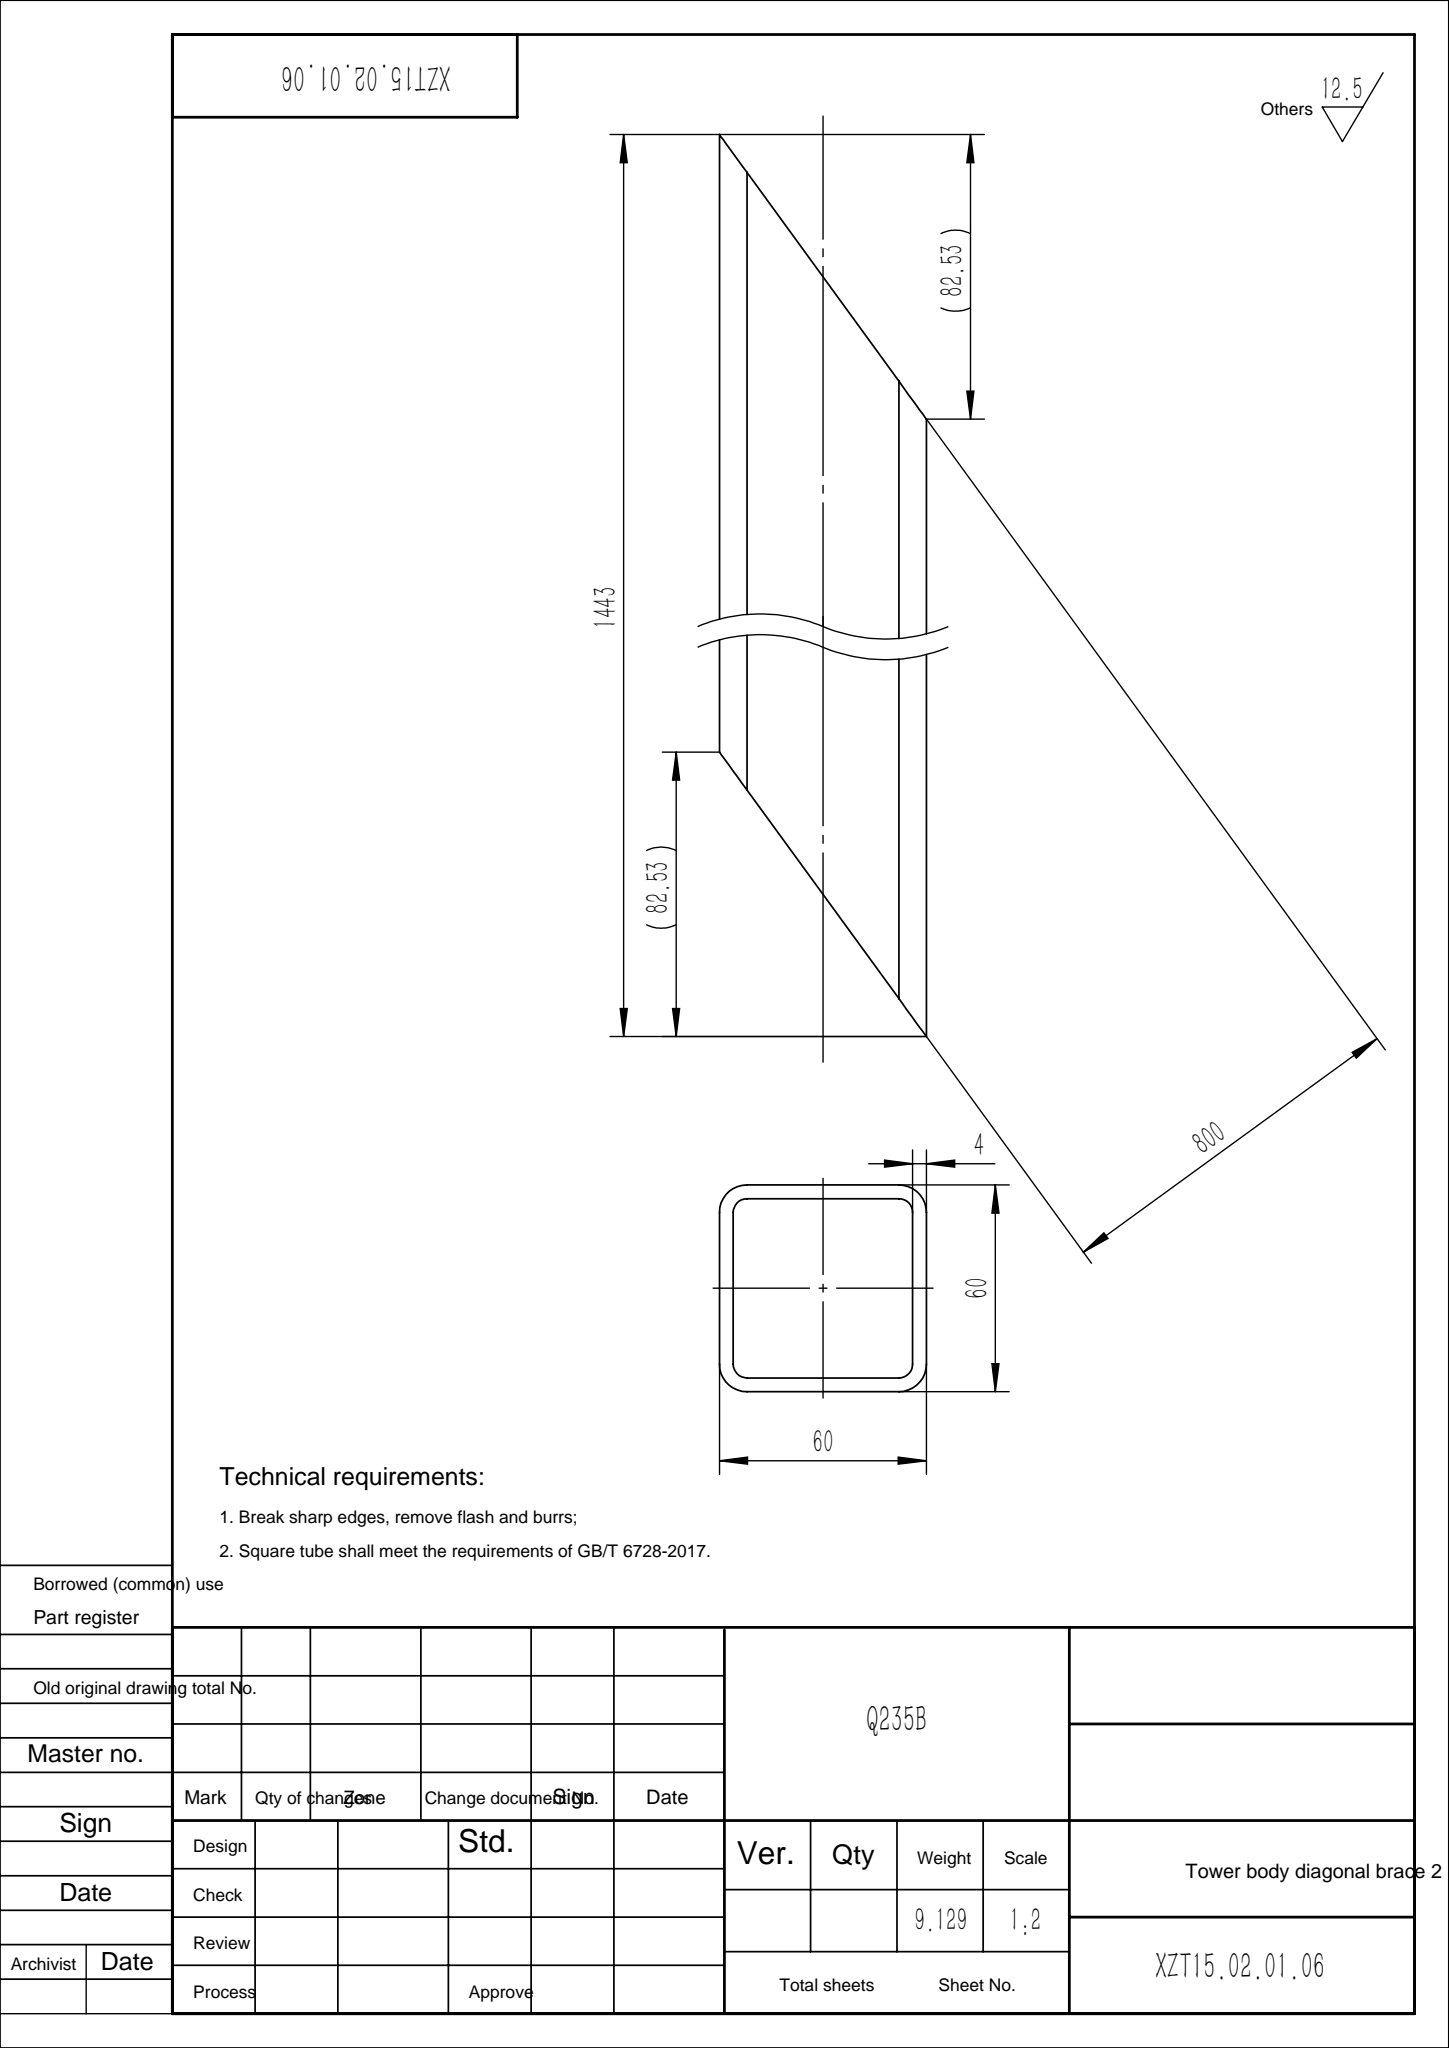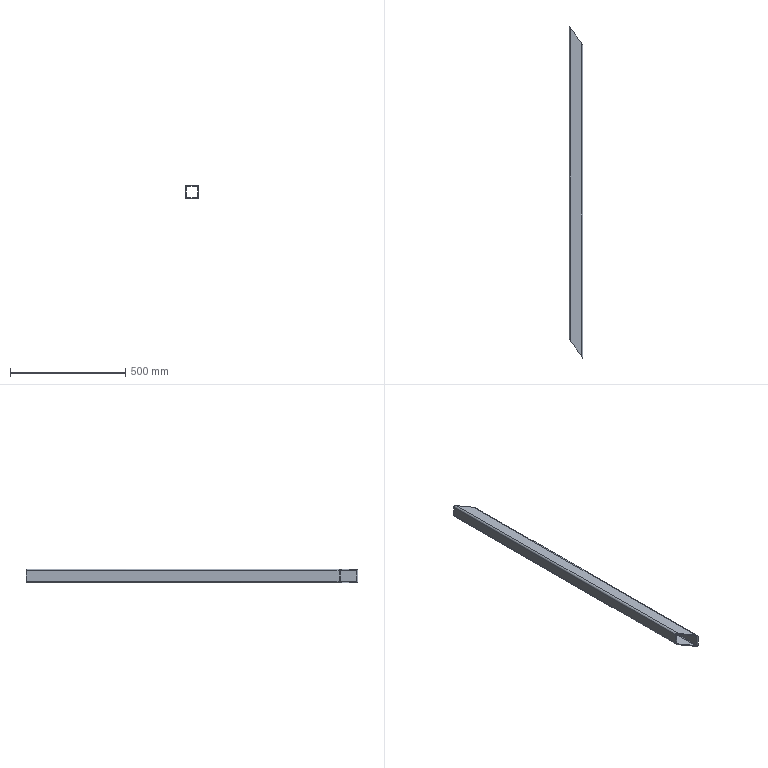Part | SolidWorks | features ICE 1, WeldMemberFeat 1, WeldmentFeature 1 | 1 solid | 18 faces | box 60 x 1443 x 60 mm | volume 1162925 mm3 | plane 10 | cylinder 8 | commonest cylinder face diameters 8 x4 16 x4
STEP:
#1=CARTESIAN_POINT('',(30.,1360.47,-22.));
#2=VERTEX_POINT('',#1);
#3=CARTESIAN_POINT('',(30.,0.,-22.));
#4=VERTEX_POINT('',#3);
#5=CARTESIAN_POINT('',(30.,1443.,-22.));
#6=DIRECTION('',(0.,-1.,0.));
#7=VECTOR('',#6,1000.);
#8=LINE('',#5,#7);
#9=EDGE_CURVE('',#2,#4,#8,.T.);
#10=ORIENTED_EDGE('',*,*,#9,.F.);
#11=CARTESIAN_POINT('',(30.,1360.47,22.));
#12=VERTEX_POINT('',#11);
#13=CARTESIAN_POINT('',(30.,1360.47,-30.));
#14=DIRECTION('',(0.,0.,1.));
#15=VECTOR('',#14,1000.);
#16=LINE('',#13,#15);
#17=EDGE_CURVE('',#2,#12,#16,.T.);
#18=ORIENTED_EDGE('',*,*,#17,.T.);
#19=CARTESIAN_POINT('',(30.,0.,22.));
#20=VERTEX_POINT('',#19);
#21=CARTESIAN_POINT('',(30.,1443.,22.));
#22=DIRECTION('',(0.,-1.,0.));
#23=VECTOR('',#22,1000.);
#24=LINE('',#21,#23);
#25=EDGE_CURVE('',#12,#20,#24,.T.);
#26=ORIENTED_EDGE('',*,*,#25,.T.);
#27=CARTESIAN_POINT('',(30.,0.,-22.));
#28=DIRECTION('',(0.,0.,-1.));
#29=VECTOR('',#28,1000.);
#30=LINE('',#27,#29);
#31=EDGE_CURVE('',#20,#4,#30,.T.);
#32=ORIENTED_EDGE('',*,*,#31,.T.);
#33=EDGE_LOOP('',(#10,#18,#26,#32));
#34=FACE_OUTER_BOUND('',#33,.T.);
#35=CARTESIAN_POINT('',(30.,1443.,-22.));
#36=DIRECTION('',(-1.,0.,0.));
#37=DIRECTION('',(0.,0.,1.));
#38=AXIS2_PLACEMENT_3D('',#35,#36,#37);
#39=PLANE('',#38);
#40=ADVANCED_FACE('',(#34),#39,.F.);
#41=CARTESIAN_POINT('',(-30.,1443.,-22.));
#42=VERTEX_POINT('',#41);
#43=CARTESIAN_POINT('',(-30.,82.53,-22.));
#44=VERTEX_POINT('',#43);
#45=CARTESIAN_POINT('',(-30.,1443.,-22.));
#46=DIRECTION('',(0.,-1.,0.));
#47=VECTOR('',#46,1000.);
#48=LINE('',#45,#47);
#49=EDGE_CURVE('',#42,#44,#48,.T.);
#50=ORIENTED_EDGE('',*,*,#49,.T.);
#51=CARTESIAN_POINT('',(-30.,82.53,22.));
#52=VERTEX_POINT('',#51);
#53=CARTESIAN_POINT('',(-30.,82.53,-30.));
#54=DIRECTION('',(0.,0.,1.));
#55=VECTOR('',#54,1000.);
#56=LINE('',#53,#55);
#57=EDGE_CURVE('',#44,#52,#56,.T.);
#58=ORIENTED_EDGE('',*,*,#57,.T.);
#59=CARTESIAN_POINT('',(-30.,1443.,22.));
#60=VERTEX_POINT('',#59);
#61=CARTESIAN_POINT('',(-30.,1443.,22.));
#62=DIRECTION('',(0.,-1.,0.));
#63=VECTOR('',#62,1000.);
#64=LINE('',#61,#63);
#65=EDGE_CURVE('',#60,#52,#64,.T.);
#66=ORIENTED_EDGE('',*,*,#65,.F.);
#67=CARTESIAN_POINT('',(-30.,1443.,22.));
#68=DIRECTION('',(0.,0.,1.));
#69=VECTOR('',#68,1000.);
#70=LINE('',#67,#69);
#71=EDGE_CURVE('',#42,#60,#70,.T.);
#72=ORIENTED_EDGE('',*,*,#71,.F.);
#73=EDGE_LOOP('',(#50,#58,#66,#72));
#74=FACE_OUTER_BOUND('',#73,.T.);
#75=CARTESIAN_POINT('',(-30.,1443.,22.));
#76=DIRECTION('',(1.,0.,0.));
#77=DIRECTION('',(0.,0.,-1.));
#78=AXIS2_PLACEMENT_3D('',#75,#76,#77);
#79=PLANE('',#78);
#80=ADVANCED_FACE('',(#74),#79,.F.);
#81=ORIENTED_EDGE('',*,*,#49,.F.);
#82=CARTESIAN_POINT('',(-22.,1431.996,-30.));
#83=VERTEX_POINT('',#82);
#84=CARTESIAN_POINT('',(-30.,1443.,-22.));
#85=CARTESIAN_POINT('',(-30.,1443.,-26.686));
#86=CARTESIAN_POINT('',(-26.686,1438.442,-30.));
#87=CARTESIAN_POINT('',(-22.,1431.996,-30.));
#88=(BOUNDED_CURVE()B_SPLINE_CURVE(3,(#84,#85,#86,#87),.UNSPECIFIED.,.F.,.F.)B_SPLINE_CURVE_WITH_KNOTS((4,4),(3.142,4.712),.UNSPECIFIED.)CURVE()GEOMETRIC_REPRESENTATION_ITEM()RATIONAL_B_SPLINE_CURVE((1.,0.8047,0.8047,1.))REPRESENTATION_ITEM(''));
#89=EDGE_CURVE('',#42,#83,#88,.T.);
#90=ORIENTED_EDGE('',*,*,#89,.T.);
#91=CARTESIAN_POINT('',(-22.,71.526,-30.));
#92=VERTEX_POINT('',#91);
#93=CARTESIAN_POINT('',(-22.,1443.,-30.));
#94=DIRECTION('',(0.,-1.,0.));
#95=VECTOR('',#94,1000.);
#96=LINE('',#93,#95);
#97=EDGE_CURVE('',#83,#92,#96,.T.);
#98=ORIENTED_EDGE('',*,*,#97,.T.);
#99=CARTESIAN_POINT('',(-22.,71.526,-30.));
#100=CARTESIAN_POINT('',(-26.686,77.972,-30.));
#101=CARTESIAN_POINT('',(-30.,82.53,-26.686));
#102=CARTESIAN_POINT('',(-30.,82.53,-22.));
#103=(BOUNDED_CURVE()B_SPLINE_CURVE(3,(#99,#100,#101,#102),.UNSPECIFIED.,.F.,.F.)B_SPLINE_CURVE_WITH_KNOTS((4,4),(1.571,3.142),.UNSPECIFIED.)CURVE()GEOMETRIC_REPRESENTATION_ITEM()RATIONAL_B_SPLINE_CURVE((1.,0.8047,0.8047,1.))REPRESENTATION_ITEM(''));
#104=EDGE_CURVE('',#92,#44,#103,.T.);
#105=ORIENTED_EDGE('',*,*,#104,.T.);
#106=EDGE_LOOP('',(#81,#90,#98,#105));
#107=FACE_OUTER_BOUND('',#106,.T.);
#108=CARTESIAN_POINT('',(-22.,1443.,-22.));
#109=DIRECTION('',(0.,-1.,0.));
#110=DIRECTION('',(0.,0.,-1.));
#111=AXIS2_PLACEMENT_3D('',#108,#109,#110);
#112=CYLINDRICAL_SURFACE('',#111,8.);
#113=ADVANCED_FACE('',(#107),#112,.T.);
#114=ORIENTED_EDGE('',*,*,#97,.F.);
#115=CARTESIAN_POINT('',(22.,1371.474,-30.));
#116=VERTEX_POINT('',#115);
#117=CARTESIAN_POINT('',(-30.,1443.,-30.));
#118=DIRECTION('',(0.588,-0.8088,0.));
#119=VECTOR('',#118,1000.);
#120=LINE('',#117,#119);
#121=EDGE_CURVE('',#83,#116,#120,.T.);
#122=ORIENTED_EDGE('',*,*,#121,.T.);
#123=CARTESIAN_POINT('',(22.,11.004,-30.));
#124=VERTEX_POINT('',#123);
#125=CARTESIAN_POINT('',(22.,1443.,-30.));
#126=DIRECTION('',(0.,-1.,0.));
#127=VECTOR('',#126,1000.);
#128=LINE('',#125,#127);
#129=EDGE_CURVE('',#116,#124,#128,.T.);
#130=ORIENTED_EDGE('',*,*,#129,.T.);
#131=CARTESIAN_POINT('',(-30.,82.53,-30.));
#132=DIRECTION('',(-0.588,0.8088,0.));
#133=VECTOR('',#132,1000.);
#134=LINE('',#131,#133);
#135=EDGE_CURVE('',#124,#92,#134,.T.);
#136=ORIENTED_EDGE('',*,*,#135,.T.);
#137=EDGE_LOOP('',(#114,#122,#130,#136));
#138=FACE_OUTER_BOUND('',#137,.T.);
#139=CARTESIAN_POINT('',(22.,1443.,-30.));
#140=DIRECTION('',(0.,0.,1.));
#141=DIRECTION('',(1.,0.,0.));
#142=AXIS2_PLACEMENT_3D('',#139,#140,#141);
#143=PLANE('',#142);
#144=ADVANCED_FACE('',(#138),#143,.F.);
#145=ORIENTED_EDGE('',*,*,#129,.F.);
#146=CARTESIAN_POINT('',(22.,1371.474,-30.));
#147=CARTESIAN_POINT('',(26.686,1365.028,-30.));
#148=CARTESIAN_POINT('',(30.,1360.47,-26.686));
#149=CARTESIAN_POINT('',(30.,1360.47,-22.));
#150=(BOUNDED_CURVE()B_SPLINE_CURVE(3,(#146,#147,#148,#149),.UNSPECIFIED.,.F.,.F.)B_SPLINE_CURVE_WITH_KNOTS((4,4),(4.712,6.283),.UNSPECIFIED.)CURVE()GEOMETRIC_REPRESENTATION_ITEM()RATIONAL_B_SPLINE_CURVE((1.,0.8047,0.8047,1.))REPRESENTATION_ITEM(''));
#151=EDGE_CURVE('',#116,#2,#150,.T.);
#152=ORIENTED_EDGE('',*,*,#151,.T.);
#153=ORIENTED_EDGE('',*,*,#9,.T.);
#154=CARTESIAN_POINT('',(30.,0.,-22.));
#155=CARTESIAN_POINT('',(30.,0.,-26.686));
#156=CARTESIAN_POINT('',(26.686,4.558,-30.));
#157=CARTESIAN_POINT('',(22.,11.004,-30.));
#158=(BOUNDED_CURVE()B_SPLINE_CURVE(3,(#154,#155,#156,#157),.UNSPECIFIED.,.F.,.F.)B_SPLINE_CURVE_WITH_KNOTS((4,4),(0.,1.571),.UNSPECIFIED.)CURVE()GEOMETRIC_REPRESENTATION_ITEM()RATIONAL_B_SPLINE_CURVE((1.,0.8047,0.8047,1.))REPRESENTATION_ITEM(''));
#159=EDGE_CURVE('',#4,#124,#158,.T.);
#160=ORIENTED_EDGE('',*,*,#159,.T.);
#161=EDGE_LOOP('',(#145,#152,#153,#160));
#162=FACE_OUTER_BOUND('',#161,.T.);
#163=CARTESIAN_POINT('',(22.,1443.,-22.));
#164=DIRECTION('',(0.,-1.,0.));
#165=DIRECTION('',(0.,0.,-1.));
#166=AXIS2_PLACEMENT_3D('',#163,#164,#165);
#167=CYLINDRICAL_SURFACE('',#166,8.);
#168=ADVANCED_FACE('',(#162),#167,.T.);
#169=ORIENTED_EDGE('',*,*,#25,.F.);
#170=CARTESIAN_POINT('',(22.,1371.474,30.));
#171=VERTEX_POINT('',#170);
#172=CARTESIAN_POINT('',(30.,1360.47,22.));
#173=CARTESIAN_POINT('',(30.,1360.47,26.686));
#174=CARTESIAN_POINT('',(26.686,1365.028,30.));
#175=CARTESIAN_POINT('',(22.,1371.474,30.));
#176=(BOUNDED_CURVE()B_SPLINE_CURVE(3,(#172,#173,#174,#175),.UNSPECIFIED.,.F.,.F.)B_SPLINE_CURVE_WITH_KNOTS((4,4),(0.,1.571),.UNSPECIFIED.)CURVE()GEOMETRIC_REPRESENTATION_ITEM()RATIONAL_B_SPLINE_CURVE((1.,0.8047,0.8047,1.))REPRESENTATION_ITEM(''));
#177=EDGE_CURVE('',#12,#171,#176,.T.);
#178=ORIENTED_EDGE('',*,*,#177,.T.);
#179=CARTESIAN_POINT('',(22.,11.004,30.));
#180=VERTEX_POINT('',#179);
#181=CARTESIAN_POINT('',(22.,1443.,30.));
#182=DIRECTION('',(0.,-1.,0.));
#183=VECTOR('',#182,1000.);
#184=LINE('',#181,#183);
#185=EDGE_CURVE('',#171,#180,#184,.T.);
#186=ORIENTED_EDGE('',*,*,#185,.T.);
#187=CARTESIAN_POINT('',(22.,11.004,30.));
#188=CARTESIAN_POINT('',(26.686,4.558,30.));
#189=CARTESIAN_POINT('',(30.,0.,26.686));
#190=CARTESIAN_POINT('',(30.,0.,22.));
#191=(BOUNDED_CURVE()B_SPLINE_CURVE(3,(#187,#188,#189,#190),.UNSPECIFIED.,.F.,.F.)B_SPLINE_CURVE_WITH_KNOTS((4,4),(4.712,6.283),.UNSPECIFIED.)CURVE()GEOMETRIC_REPRESENTATION_ITEM()RATIONAL_B_SPLINE_CURVE((1.,0.8047,0.8047,1.))REPRESENTATION_ITEM(''));
#192=EDGE_CURVE('',#180,#20,#191,.T.);
#193=ORIENTED_EDGE('',*,*,#192,.T.);
#194=EDGE_LOOP('',(#169,#178,#186,#193));
#195=FACE_OUTER_BOUND('',#194,.T.);
#196=CARTESIAN_POINT('',(22.,1443.,22.));
#197=DIRECTION('',(0.,-1.,0.));
#198=DIRECTION('',(0.,0.,-1.));
#199=AXIS2_PLACEMENT_3D('',#196,#197,#198);
#200=CYLINDRICAL_SURFACE('',#199,8.);
#201=ADVANCED_FACE('',(#195),#200,.T.);
#202=ORIENTED_EDGE('',*,*,#185,.F.);
#203=CARTESIAN_POINT('',(-22.,1431.996,30.));
#204=VERTEX_POINT('',#203);
#205=CARTESIAN_POINT('',(-27.234,1439.195,30.));
#206=DIRECTION('',(-0.588,0.8088,0.));
#207=VECTOR('',#206,1000.);
#208=LINE('',#205,#207);
#209=EDGE_CURVE('',#171,#204,#208,.T.);
#210=ORIENTED_EDGE('',*,*,#209,.T.);
#211=CARTESIAN_POINT('',(-22.,71.526,30.));
#212=VERTEX_POINT('',#211);
#213=CARTESIAN_POINT('',(-22.,1443.,30.));
#214=DIRECTION('',(0.,-1.,0.));
#215=VECTOR('',#214,1000.);
#216=LINE('',#213,#215);
#217=EDGE_CURVE('',#204,#212,#216,.T.);
#218=ORIENTED_EDGE('',*,*,#217,.T.);
#219=CARTESIAN_POINT('',(-674.304,968.769,30.));
#220=DIRECTION('',(0.588,-0.8088,0.));
#221=VECTOR('',#220,1000.);
#222=LINE('',#219,#221);
#223=EDGE_CURVE('',#212,#180,#222,.T.);
#224=ORIENTED_EDGE('',*,*,#223,.T.);
#225=EDGE_LOOP('',(#202,#210,#218,#224));
#226=FACE_OUTER_BOUND('',#225,.T.);
#227=CARTESIAN_POINT('',(-22.,1443.,30.));
#228=DIRECTION('',(0.,0.,-1.));
#229=DIRECTION('',(-1.,0.,0.));
#230=AXIS2_PLACEMENT_3D('',#227,#228,#229);
#231=PLANE('',#230);
#232=ADVANCED_FACE('',(#226),#231,.F.);
#233=ORIENTED_EDGE('',*,*,#217,.F.);
#234=CARTESIAN_POINT('',(-22.,1431.996,30.));
#235=CARTESIAN_POINT('',(-26.686,1438.442,30.));
#236=CARTESIAN_POINT('',(-30.,1443.,26.686));
#237=CARTESIAN_POINT('',(-30.,1443.,22.));
#238=(BOUNDED_CURVE()B_SPLINE_CURVE(3,(#234,#235,#236,#237),.UNSPECIFIED.,.F.,.F.)B_SPLINE_CURVE_WITH_KNOTS((4,4),(1.571,3.142),.UNSPECIFIED.)CURVE()GEOMETRIC_REPRESENTATION_ITEM()RATIONAL_B_SPLINE_CURVE((1.,0.8047,0.8047,1.))REPRESENTATION_ITEM(''));
#239=EDGE_CURVE('',#204,#60,#238,.T.);
#240=ORIENTED_EDGE('',*,*,#239,.T.);
#241=ORIENTED_EDGE('',*,*,#65,.T.);
#242=CARTESIAN_POINT('',(-30.,82.53,22.));
#243=CARTESIAN_POINT('',(-30.,82.53,26.686));
#244=CARTESIAN_POINT('',(-26.686,77.972,30.));
#245=CARTESIAN_POINT('',(-22.,71.526,30.));
#246=(BOUNDED_CURVE()B_SPLINE_CURVE(3,(#242,#243,#244,#245),.UNSPECIFIED.,.F.,.F.)B_SPLINE_CURVE_WITH_KNOTS((4,4),(3.142,4.712),.UNSPECIFIED.)CURVE()GEOMETRIC_REPRESENTATION_ITEM()RATIONAL_B_SPLINE_CURVE((1.,0.8047,0.8047,1.))REPRESENTATION_ITEM(''));
#247=EDGE_CURVE('',#52,#212,#246,.T.);
#248=ORIENTED_EDGE('',*,*,#247,.T.);
#249=EDGE_LOOP('',(#233,#240,#241,#248));
#250=FACE_OUTER_BOUND('',#249,.T.);
#251=CARTESIAN_POINT('',(-22.,1443.,22.));
#252=DIRECTION('',(0.,-1.,0.));
#253=DIRECTION('',(0.,0.,-1.));
#254=AXIS2_PLACEMENT_3D('',#251,#252,#253);
#255=CYLINDRICAL_SURFACE('',#254,8.);
#256=ADVANCED_FACE('',(#250),#255,.T.);
#257=CARTESIAN_POINT('',(22.,11.004,26.));
#258=VERTEX_POINT('',#257);
#259=CARTESIAN_POINT('',(26.,5.502,22.));
#260=VERTEX_POINT('',#259);
#261=CARTESIAN_POINT('',(22.,11.004,26.));
#262=CARTESIAN_POINT('',(24.343,7.781,26.));
#263=CARTESIAN_POINT('',(26.,5.502,24.343));
#264=CARTESIAN_POINT('',(26.,5.502,22.));
#265=(BOUNDED_CURVE()B_SPLINE_CURVE(3,(#261,#262,#263,#264),.UNSPECIFIED.,.F.,.F.)B_SPLINE_CURVE_WITH_KNOTS((4,4),(4.712,6.283),.UNSPECIFIED.)CURVE()GEOMETRIC_REPRESENTATION_ITEM()RATIONAL_B_SPLINE_CURVE((1.,0.8047,0.8047,1.))REPRESENTATION_ITEM(''));
#266=EDGE_CURVE('',#258,#260,#265,.T.);
#267=ORIENTED_EDGE('',*,*,#266,.T.);
#268=CARTESIAN_POINT('',(26.,5.502,-22.));
#269=VERTEX_POINT('',#268);
#270=CARTESIAN_POINT('',(26.,5.502,-22.));
#271=DIRECTION('',(0.,0.,-1.));
#272=VECTOR('',#271,1000.);
#273=LINE('',#270,#272);
#274=EDGE_CURVE('',#260,#269,#273,.T.);
#275=ORIENTED_EDGE('',*,*,#274,.T.);
#276=CARTESIAN_POINT('',(22.,11.004,-26.));
#277=VERTEX_POINT('',#276);
#278=CARTESIAN_POINT('',(26.,5.502,-22.));
#279=CARTESIAN_POINT('',(26.,5.502,-24.343));
#280=CARTESIAN_POINT('',(24.343,7.781,-26.));
#281=CARTESIAN_POINT('',(22.,11.004,-26.));
#282=(BOUNDED_CURVE()B_SPLINE_CURVE(3,(#278,#279,#280,#281),.UNSPECIFIED.,.F.,.F.)B_SPLINE_CURVE_WITH_KNOTS((4,4),(0.,1.571),.UNSPECIFIED.)CURVE()GEOMETRIC_REPRESENTATION_ITEM()RATIONAL_B_SPLINE_CURVE((1.,0.8047,0.8047,1.))REPRESENTATION_ITEM(''));
#283=EDGE_CURVE('',#269,#277,#282,.T.);
#284=ORIENTED_EDGE('',*,*,#283,.T.);
#285=CARTESIAN_POINT('',(-22.,71.526,-26.));
#286=VERTEX_POINT('',#285);
#287=CARTESIAN_POINT('',(-659.089,947.842,-26.));
#288=DIRECTION('',(-0.588,0.8088,0.));
#289=VECTOR('',#288,1000.);
#290=LINE('',#287,#289);
#291=EDGE_CURVE('',#277,#286,#290,.T.);
#292=ORIENTED_EDGE('',*,*,#291,.T.);
#293=CARTESIAN_POINT('',(-26.,77.028,-22.));
#294=VERTEX_POINT('',#293);
#295=CARTESIAN_POINT('',(-22.,71.526,-26.));
#296=CARTESIAN_POINT('',(-24.343,74.749,-26.));
#297=CARTESIAN_POINT('',(-26.,77.028,-24.343));
#298=CARTESIAN_POINT('',(-26.,77.028,-22.));
#299=(BOUNDED_CURVE()B_SPLINE_CURVE(3,(#295,#296,#297,#298),.UNSPECIFIED.,.F.,.F.)B_SPLINE_CURVE_WITH_KNOTS((4,4),(1.571,3.142),.UNSPECIFIED.)CURVE()GEOMETRIC_REPRESENTATION_ITEM()RATIONAL_B_SPLINE_CURVE((1.,0.8047,0.8047,1.))REPRESENTATION_ITEM(''));
#300=EDGE_CURVE('',#286,#294,#299,.T.);
#301=ORIENTED_EDGE('',*,*,#300,.T.);
#302=CARTESIAN_POINT('',(-26.,77.028,22.));
#303=VERTEX_POINT('',#302);
#304=CARTESIAN_POINT('',(-26.,77.028,22.));
#305=DIRECTION('',(0.,0.,1.));
#306=VECTOR('',#305,1000.);
#307=LINE('',#304,#306);
#308=EDGE_CURVE('',#294,#303,#307,.T.);
#309=ORIENTED_EDGE('',*,*,#308,.T.);
#310=CARTESIAN_POINT('',(-22.,71.526,26.));
#311=VERTEX_POINT('',#310);
#312=CARTESIAN_POINT('',(-26.,77.028,22.));
#313=CARTESIAN_POINT('',(-26.,77.028,24.343));
#314=CARTESIAN_POINT('',(-24.343,74.749,26.));
#315=CARTESIAN_POINT('',(-22.,71.526,26.));
#316=(BOUNDED_CURVE()B_SPLINE_CURVE(3,(#312,#313,#314,#315),.UNSPECIFIED.,.F.,.T.)B_SPLINE_CURVE_WITH_KNOTS((4,4),(3.142,4.712),.UNSPECIFIED.)CURVE()GEOMETRIC_REPRESENTATION_ITEM()RATIONAL_B_SPLINE_CURVE((1.,0.8047,0.8047,1.))REPRESENTATION_ITEM(''));
#317=EDGE_CURVE('',#303,#311,#316,.T.);
#318=ORIENTED_EDGE('',*,*,#317,.T.);
#319=CARTESIAN_POINT('',(-674.304,968.769,26.));
#320=DIRECTION('',(0.588,-0.8088,0.));
#321=VECTOR('',#320,1000.);
#322=LINE('',#319,#321);
#323=EDGE_CURVE('',#311,#258,#322,.T.);
#324=ORIENTED_EDGE('',*,*,#323,.T.);
#325=EDGE_LOOP('',(#267,#275,#284,#292,#301,#309,#318,#324));
#326=FACE_BOUND('',#325,.T.);
#327=ORIENTED_EDGE('',*,*,#57,.F.);
#328=ORIENTED_EDGE('',*,*,#104,.F.);
#329=ORIENTED_EDGE('',*,*,#135,.F.);
#330=ORIENTED_EDGE('',*,*,#159,.F.);
#331=ORIENTED_EDGE('',*,*,#31,.F.);
#332=ORIENTED_EDGE('',*,*,#192,.F.);
#333=ORIENTED_EDGE('',*,*,#223,.F.);
#334=ORIENTED_EDGE('',*,*,#247,.F.);
#335=EDGE_LOOP('',(#327,#328,#329,#330,#331,#332,#333,#334));
#336=FACE_OUTER_BOUND('',#335,.T.);
#337=CARTESIAN_POINT('',(-30.,82.53,-30.));
#338=DIRECTION('',(0.8088,0.588,0.));
#339=DIRECTION('',(-0.588,0.8088,0.));
#340=AXIS2_PLACEMENT_3D('',#337,#338,#339);
#341=PLANE('',#340);
#342=ADVANCED_FACE('',(#326,#336),#341,.F.);
#343=CARTESIAN_POINT('',(26.,1365.972,22.));
#344=VERTEX_POINT('',#343);
#345=CARTESIAN_POINT('',(22.,1371.474,26.));
#346=VERTEX_POINT('',#345);
#347=CARTESIAN_POINT('',(26.,1365.972,22.));
#348=CARTESIAN_POINT('',(26.,1365.972,24.343));
#349=CARTESIAN_POINT('',(24.343,1368.251,26.));
#350=CARTESIAN_POINT('',(22.,1371.474,26.));
#351=(BOUNDED_CURVE()B_SPLINE_CURVE(3,(#347,#348,#349,#350),.UNSPECIFIED.,.F.,.F.)B_SPLINE_CURVE_WITH_KNOTS((4,4),(0.,1.571),.UNSPECIFIED.)CURVE()GEOMETRIC_REPRESENTATION_ITEM()RATIONAL_B_SPLINE_CURVE((1.,0.8047,0.8047,1.))REPRESENTATION_ITEM(''));
#352=EDGE_CURVE('',#344,#346,#351,.T.);
#353=ORIENTED_EDGE('',*,*,#352,.T.);
#354=CARTESIAN_POINT('',(-22.,1431.996,26.));
#355=VERTEX_POINT('',#354);
#356=CARTESIAN_POINT('',(-27.234,1439.195,26.));
#357=DIRECTION('',(-0.588,0.8088,0.));
#358=VECTOR('',#357,1000.);
#359=LINE('',#356,#358);
#360=EDGE_CURVE('',#346,#355,#359,.T.);
#361=ORIENTED_EDGE('',*,*,#360,.T.);
#362=CARTESIAN_POINT('',(-26.,1437.498,22.));
#363=VERTEX_POINT('',#362);
#364=CARTESIAN_POINT('',(-22.,1431.996,26.));
#365=CARTESIAN_POINT('',(-24.343,1435.219,26.));
#366=CARTESIAN_POINT('',(-26.,1437.498,24.343));
#367=CARTESIAN_POINT('',(-26.,1437.498,22.));
#368=(BOUNDED_CURVE()B_SPLINE_CURVE(3,(#364,#365,#366,#367),.UNSPECIFIED.,.F.,.F.)B_SPLINE_CURVE_WITH_KNOTS((4,4),(1.571,3.142),.UNSPECIFIED.)CURVE()GEOMETRIC_REPRESENTATION_ITEM()RATIONAL_B_SPLINE_CURVE((1.,0.8047,0.8047,1.))REPRESENTATION_ITEM(''));
#369=EDGE_CURVE('',#355,#363,#368,.T.);
#370=ORIENTED_EDGE('',*,*,#369,.T.);
#371=CARTESIAN_POINT('',(-26.,1437.498,-22.));
#372=VERTEX_POINT('',#371);
#373=CARTESIAN_POINT('',(-26.,1437.498,22.));
#374=DIRECTION('',(0.,0.,-1.));
#375=VECTOR('',#374,1000.);
#376=LINE('',#373,#375);
#377=EDGE_CURVE('',#363,#372,#376,.T.);
#378=ORIENTED_EDGE('',*,*,#377,.T.);
#379=CARTESIAN_POINT('',(-22.,1431.996,-26.));
#380=VERTEX_POINT('',#379);
#381=CARTESIAN_POINT('',(-26.,1437.498,-22.));
#382=CARTESIAN_POINT('',(-26.,1437.498,-24.343));
#383=CARTESIAN_POINT('',(-24.343,1435.219,-26.));
#384=CARTESIAN_POINT('',(-22.,1431.996,-26.));
#385=(BOUNDED_CURVE()B_SPLINE_CURVE(3,(#381,#382,#383,#384),.UNSPECIFIED.,.F.,.F.)B_SPLINE_CURVE_WITH_KNOTS((4,4),(3.142,4.712),.UNSPECIFIED.)CURVE()GEOMETRIC_REPRESENTATION_ITEM()RATIONAL_B_SPLINE_CURVE((1.,0.8047,0.8047,1.))REPRESENTATION_ITEM(''));
#386=EDGE_CURVE('',#372,#380,#385,.T.);
#387=ORIENTED_EDGE('',*,*,#386,.T.);
#388=CARTESIAN_POINT('',(22.,1371.474,-26.));
#389=VERTEX_POINT('',#388);
#390=CARTESIAN_POINT('',(-12.019,1418.268,-26.));
#391=DIRECTION('',(0.588,-0.8088,0.));
#392=VECTOR('',#391,1000.);
#393=LINE('',#390,#392);
#394=EDGE_CURVE('',#380,#389,#393,.T.);
#395=ORIENTED_EDGE('',*,*,#394,.T.);
#396=CARTESIAN_POINT('',(26.,1365.972,-22.));
#397=VERTEX_POINT('',#396);
#398=CARTESIAN_POINT('',(22.,1371.474,-26.));
#399=CARTESIAN_POINT('',(24.343,1368.251,-26.));
#400=CARTESIAN_POINT('',(26.,1365.972,-24.343));
#401=CARTESIAN_POINT('',(26.,1365.972,-22.));
#402=(BOUNDED_CURVE()B_SPLINE_CURVE(3,(#398,#399,#400,#401),.UNSPECIFIED.,.F.,.F.)B_SPLINE_CURVE_WITH_KNOTS((4,4),(4.712,6.283),.UNSPECIFIED.)CURVE()GEOMETRIC_REPRESENTATION_ITEM()RATIONAL_B_SPLINE_CURVE((1.,0.8047,0.8047,1.))REPRESENTATION_ITEM(''));
#403=EDGE_CURVE('',#389,#397,#402,.T.);
#404=ORIENTED_EDGE('',*,*,#403,.T.);
#405=CARTESIAN_POINT('',(26.,1365.972,-22.));
#406=DIRECTION('',(0.,0.,1.));
#407=VECTOR('',#406,1000.);
#408=LINE('',#405,#407);
#409=EDGE_CURVE('',#397,#344,#408,.T.);
#410=ORIENTED_EDGE('',*,*,#409,.T.);
#411=EDGE_LOOP('',(#353,#361,#370,#378,#387,#395,#404,#410));
#412=FACE_BOUND('',#411,.T.);
#413=ORIENTED_EDGE('',*,*,#209,.F.);
#414=ORIENTED_EDGE('',*,*,#177,.F.);
#415=ORIENTED_EDGE('',*,*,#17,.F.);
#416=ORIENTED_EDGE('',*,*,#151,.F.);
#417=ORIENTED_EDGE('',*,*,#121,.F.);
#418=ORIENTED_EDGE('',*,*,#89,.F.);
#419=ORIENTED_EDGE('',*,*,#71,.T.);
#420=ORIENTED_EDGE('',*,*,#239,.F.);
#421=EDGE_LOOP('',(#413,#414,#415,#416,#417,#418,#419,#420));
#422=FACE_OUTER_BOUND('',#421,.T.);
#423=CARTESIAN_POINT('',(-30.,1443.,-30.));
#424=DIRECTION('',(-0.8088,-0.588,0.));
#425=DIRECTION('',(0.588,-0.8088,0.));
#426=AXIS2_PLACEMENT_3D('',#423,#424,#425);
#427=PLANE('',#426);
#428=ADVANCED_FACE('',(#412,#422),#427,.F.);
#429=ORIENTED_EDGE('',*,*,#352,.F.);
#430=CARTESIAN_POINT('',(26.,1443.,22.));
#431=DIRECTION('',(0.,-1.,0.));
#432=VECTOR('',#431,1000.);
#433=LINE('',#430,#432);
#434=EDGE_CURVE('',#344,#260,#433,.T.);
#435=ORIENTED_EDGE('',*,*,#434,.T.);
#436=ORIENTED_EDGE('',*,*,#266,.F.);
#437=CARTESIAN_POINT('',(22.,1443.,26.));
#438=DIRECTION('',(0.,-1.,0.));
#439=VECTOR('',#438,1000.);
#440=LINE('',#437,#439);
#441=EDGE_CURVE('',#346,#258,#440,.T.);
#442=ORIENTED_EDGE('',*,*,#441,.F.);
#443=EDGE_LOOP('',(#429,#435,#436,#442));
#444=FACE_OUTER_BOUND('',#443,.T.);
#445=CARTESIAN_POINT('',(22.,1443.,22.));
#446=DIRECTION('',(0.,-1.,0.));
#447=DIRECTION('',(0.,0.,-1.));
#448=AXIS2_PLACEMENT_3D('',#445,#446,#447);
#449=CYLINDRICAL_SURFACE('',#448,4.);
#450=ADVANCED_FACE('',(#444),#449,.F.);
#451=ORIENTED_EDGE('',*,*,#360,.F.);
#452=ORIENTED_EDGE('',*,*,#441,.T.);
#453=ORIENTED_EDGE('',*,*,#323,.F.);
#454=CARTESIAN_POINT('',(-22.,1443.,26.));
#455=DIRECTION('',(0.,-1.,0.));
#456=VECTOR('',#455,1000.);
#457=LINE('',#454,#456);
#458=EDGE_CURVE('',#355,#311,#457,.T.);
#459=ORIENTED_EDGE('',*,*,#458,.F.);
#460=EDGE_LOOP('',(#451,#452,#453,#459));
#461=FACE_OUTER_BOUND('',#460,.T.);
#462=CARTESIAN_POINT('',(-22.,1443.,26.));
#463=DIRECTION('',(0.,0.,-1.));
#464=DIRECTION('',(-1.,0.,0.));
#465=AXIS2_PLACEMENT_3D('',#462,#463,#464);
#466=PLANE('',#465);
#467=ADVANCED_FACE('',(#461),#466,.T.);
#468=ORIENTED_EDGE('',*,*,#369,.F.);
#469=ORIENTED_EDGE('',*,*,#458,.T.);
#470=ORIENTED_EDGE('',*,*,#317,.F.);
#471=CARTESIAN_POINT('',(-26.,1443.,22.));
#472=DIRECTION('',(0.,-1.,0.));
#473=VECTOR('',#472,1000.);
#474=LINE('',#471,#473);
#475=EDGE_CURVE('',#363,#303,#474,.T.);
#476=ORIENTED_EDGE('',*,*,#475,.F.);
#477=EDGE_LOOP('',(#468,#469,#470,#476));
#478=FACE_OUTER_BOUND('',#477,.T.);
#479=CARTESIAN_POINT('',(-22.,1443.,22.));
#480=DIRECTION('',(0.,-1.,0.));
#481=DIRECTION('',(0.,0.,-1.));
#482=AXIS2_PLACEMENT_3D('',#479,#480,#481);
#483=CYLINDRICAL_SURFACE('',#482,4.);
#484=ADVANCED_FACE('',(#478),#483,.F.);
#485=ORIENTED_EDGE('',*,*,#377,.F.);
#486=ORIENTED_EDGE('',*,*,#475,.T.);
#487=ORIENTED_EDGE('',*,*,#308,.F.);
#488=CARTESIAN_POINT('',(-26.,1443.,-22.));
#489=DIRECTION('',(0.,-1.,0.));
#490=VECTOR('',#489,1000.);
#491=LINE('',#488,#490);
#492=EDGE_CURVE('',#372,#294,#491,.T.);
#493=ORIENTED_EDGE('',*,*,#492,.F.);
#494=EDGE_LOOP('',(#485,#486,#487,#493));
#495=FACE_OUTER_BOUND('',#494,.T.);
#496=CARTESIAN_POINT('',(-26.,1443.,22.));
#497=DIRECTION('',(1.,0.,0.));
#498=DIRECTION('',(0.,0.,-1.));
#499=AXIS2_PLACEMENT_3D('',#496,#497,#498);
#500=PLANE('',#499);
#501=ADVANCED_FACE('',(#495),#500,.T.);
#502=ORIENTED_EDGE('',*,*,#386,.F.);
#503=ORIENTED_EDGE('',*,*,#492,.T.);
#504=ORIENTED_EDGE('',*,*,#300,.F.);
#505=CARTESIAN_POINT('',(-22.,1443.,-26.));
#506=DIRECTION('',(0.,-1.,0.));
#507=VECTOR('',#506,1000.);
#508=LINE('',#505,#507);
#509=EDGE_CURVE('',#380,#286,#508,.T.);
#510=ORIENTED_EDGE('',*,*,#509,.F.);
#511=EDGE_LOOP('',(#502,#503,#504,#510));
#512=FACE_OUTER_BOUND('',#511,.T.);
#513=CARTESIAN_POINT('',(-22.,1443.,-22.));
#514=DIRECTION('',(0.,-1.,0.));
#515=DIRECTION('',(0.,0.,-1.));
#516=AXIS2_PLACEMENT_3D('',#513,#514,#515);
#517=CYLINDRICAL_SURFACE('',#516,4.);
#518=ADVANCED_FACE('',(#512),#517,.F.);
#519=ORIENTED_EDGE('',*,*,#394,.F.);
#520=ORIENTED_EDGE('',*,*,#509,.T.);
#521=ORIENTED_EDGE('',*,*,#291,.F.);
#522=CARTESIAN_POINT('',(22.,1443.,-26.));
#523=DIRECTION('',(0.,-1.,0.));
#524=VECTOR('',#523,1000.);
#525=LINE('',#522,#524);
#526=EDGE_CURVE('',#389,#277,#525,.T.);
#527=ORIENTED_EDGE('',*,*,#526,.F.);
#528=EDGE_LOOP('',(#519,#520,#521,#527));
#529=FACE_OUTER_BOUND('',#528,.T.);
#530=CARTESIAN_POINT('',(22.,1443.,-26.));
#531=DIRECTION('',(0.,0.,1.));
#532=DIRECTION('',(1.,0.,0.));
#533=AXIS2_PLACEMENT_3D('',#530,#531,#532);
#534=PLANE('',#533);
#535=ADVANCED_FACE('',(#529),#534,.T.);
#536=ORIENTED_EDGE('',*,*,#403,.F.);
#537=ORIENTED_EDGE('',*,*,#526,.T.);
#538=ORIENTED_EDGE('',*,*,#283,.F.);
#539=CARTESIAN_POINT('',(26.,1443.,-22.));
#540=DIRECTION('',(0.,-1.,0.));
#541=VECTOR('',#540,1000.);
#542=LINE('',#539,#541);
#543=EDGE_CURVE('',#397,#269,#542,.T.);
#544=ORIENTED_EDGE('',*,*,#543,.F.);
#545=EDGE_LOOP('',(#536,#537,#538,#544));
#546=FACE_OUTER_BOUND('',#545,.T.);
#547=CARTESIAN_POINT('',(22.,1443.,-22.));
#548=DIRECTION('',(0.,-1.,0.));
#549=DIRECTION('',(0.,0.,-1.));
#550=AXIS2_PLACEMENT_3D('',#547,#548,#549);
#551=CYLINDRICAL_SURFACE('',#550,4.);
#552=ADVANCED_FACE('',(#546),#551,.F.);
#553=ORIENTED_EDGE('',*,*,#409,.F.);
#554=ORIENTED_EDGE('',*,*,#543,.T.);
#555=ORIENTED_EDGE('',*,*,#274,.F.);
#556=ORIENTED_EDGE('',*,*,#434,.F.);
#557=EDGE_LOOP('',(#553,#554,#555,#556));
#558=FACE_OUTER_BOUND('',#557,.T.);
#559=CARTESIAN_POINT('',(26.,1443.,-22.));
#560=DIRECTION('',(-1.,0.,0.));
#561=DIRECTION('',(0.,0.,1.));
#562=AXIS2_PLACEMENT_3D('',#559,#560,#561);
#563=PLANE('',#562);
#564=ADVANCED_FACE('',(#558),#563,.T.);
#565=CLOSED_SHELL('',(#40,#80,#113,#144,#168,#201,#232,#256,#342,#428,#450,#467,#484,#501,#518,#535,#552,#564));
#566=MANIFOLD_SOLID_BREP('',#565);
#567=CARTESIAN_POINT('',(0.,0.,0.));
#568=DIRECTION('',(0.,0.,1.));
#569=DIRECTION('',(1.,0.,0.));
#570=AXIS2_PLACEMENT_3D('',#567,#568,#569);
#571=(LENGTH_UNIT()NAMED_UNIT(*)SI_UNIT(.MILLI.,.METRE.));
#572=UNCERTAINTY_MEASURE_WITH_UNIT(LENGTH_MEASURE(0.00001),#571,'','');
#573=(NAMED_UNIT(*)PLANE_ANGLE_UNIT()SI_UNIT($,.RADIAN.));
#574=(NAMED_UNIT(*)SI_UNIT($,.STERADIAN.)SOLID_ANGLE_UNIT());
#575=(GEOMETRIC_REPRESENTATION_CONTEXT(3)GLOBAL_UNCERTAINTY_ASSIGNED_CONTEXT((#572))GLOBAL_UNIT_ASSIGNED_CONTEXT((#571,#573,#574))REPRESENTATION_CONTEXT('',''));
#576=ADVANCED_BREP_SHAPE_REPRESENTATION('',(#566,#570),#575);